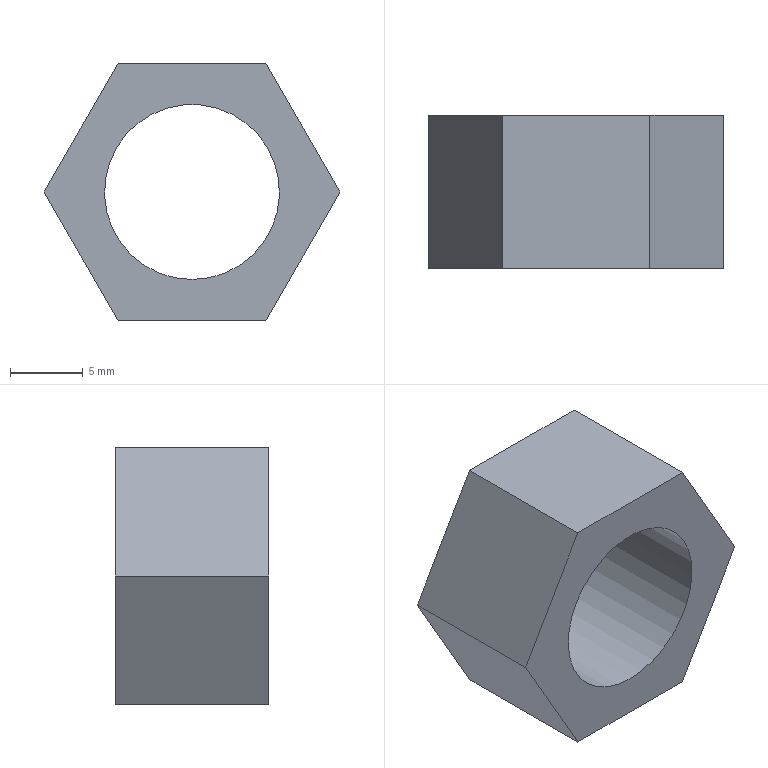Part | NX | features solid 2 | 1 solid | 9 faces | box 20.288 x 10.5 x 17.57 mm | volume 1620 mm3 | plane 8 | cylinder 1 | commonest cylinder face diameters 12 x1
STEP:
#1=CARTESIAN_POINT('',(454.928,470.5,-16.215));
#2=VERTEX_POINT('',#1);
#3=CARTESIAN_POINT('',(449.856,470.5,-25.));
#4=VERTEX_POINT('',#3);
#5=CARTESIAN_POINT('',(454.928,470.5,-16.215));
#6=DIRECTION('',(-0.5,0.,-0.866));
#7=VECTOR('',#6,1000.);
#8=LINE('',#5,#7);
#9=EDGE_CURVE('',#2,#4,#8,.T.);
#10=ORIENTED_EDGE('',*,*,#9,.F.);
#11=CARTESIAN_POINT('',(454.928,481.,-16.215));
#12=VERTEX_POINT('',#11);
#13=CARTESIAN_POINT('',(454.928,481.,-16.215));
#14=DIRECTION('',(0.,-1.,0.));
#15=VECTOR('',#14,1000.);
#16=LINE('',#13,#15);
#17=EDGE_CURVE('',#12,#2,#16,.T.);
#18=ORIENTED_EDGE('',*,*,#17,.F.);
#19=CARTESIAN_POINT('',(449.856,481.,-25.));
#20=VERTEX_POINT('',#19);
#21=CARTESIAN_POINT('',(454.928,481.,-16.215));
#22=DIRECTION('',(-0.5,0.,-0.866));
#23=VECTOR('',#22,1000.);
#24=LINE('',#21,#23);
#25=EDGE_CURVE('',#12,#20,#24,.T.);
#26=ORIENTED_EDGE('',*,*,#25,.T.);
#27=CARTESIAN_POINT('',(449.856,481.,-25.));
#28=DIRECTION('',(0.,-1.,0.));
#29=VECTOR('',#28,1000.);
#30=LINE('',#27,#29);
#31=EDGE_CURVE('',#20,#4,#30,.T.);
#32=ORIENTED_EDGE('',*,*,#31,.T.);
#33=EDGE_LOOP('',(#10,#18,#26,#32));
#34=FACE_BOUND('',#33,.T.);
#35=CARTESIAN_POINT('',(454.928,481.,-16.215));
#36=DIRECTION('',(0.866,0.,-0.5));
#37=DIRECTION('',(0.5,0.,0.866));
#38=AXIS2_PLACEMENT_3D('',#35,#36,#37);
#39=PLANE('',#38);
#40=ADVANCED_FACE('',(#34),#39,.F.);
#41=CARTESIAN_POINT('',(454.928,470.5,-33.785));
#42=VERTEX_POINT('',#41);
#43=CARTESIAN_POINT('',(449.856,470.5,-25.));
#44=DIRECTION('',(0.5,0.,-0.866));
#45=VECTOR('',#44,1000.);
#46=LINE('',#43,#45);
#47=EDGE_CURVE('',#4,#42,#46,.T.);
#48=ORIENTED_EDGE('',*,*,#47,.F.);
#49=ORIENTED_EDGE('',*,*,#31,.F.);
#50=CARTESIAN_POINT('',(454.928,481.,-33.785));
#51=VERTEX_POINT('',#50);
#52=CARTESIAN_POINT('',(449.856,481.,-25.));
#53=DIRECTION('',(0.5,0.,-0.866));
#54=VECTOR('',#53,1000.);
#55=LINE('',#52,#54);
#56=EDGE_CURVE('',#20,#51,#55,.T.);
#57=ORIENTED_EDGE('',*,*,#56,.T.);
#58=CARTESIAN_POINT('',(454.928,481.,-33.785));
#59=DIRECTION('',(0.,-1.,0.));
#60=VECTOR('',#59,1000.);
#61=LINE('',#58,#60);
#62=EDGE_CURVE('',#51,#42,#61,.T.);
#63=ORIENTED_EDGE('',*,*,#62,.T.);
#64=EDGE_LOOP('',(#48,#49,#57,#63));
#65=FACE_BOUND('',#64,.T.);
#66=CARTESIAN_POINT('',(449.856,481.,-25.));
#67=DIRECTION('',(0.866,0.,0.5));
#68=DIRECTION('',(-0.5,0.,0.866));
#69=AXIS2_PLACEMENT_3D('',#66,#67,#68);
#70=PLANE('',#69);
#71=ADVANCED_FACE('',(#65),#70,.F.);
#72=CARTESIAN_POINT('',(465.072,470.5,-33.785));
#73=VERTEX_POINT('',#72);
#74=CARTESIAN_POINT('',(454.928,470.5,-33.785));
#75=DIRECTION('',(1.,0.,0.));
#76=VECTOR('',#75,1000.);
#77=LINE('',#74,#76);
#78=EDGE_CURVE('',#42,#73,#77,.T.);
#79=ORIENTED_EDGE('',*,*,#78,.F.);
#80=ORIENTED_EDGE('',*,*,#62,.F.);
#81=CARTESIAN_POINT('',(465.072,481.,-33.785));
#82=VERTEX_POINT('',#81);
#83=CARTESIAN_POINT('',(454.928,481.,-33.785));
#84=DIRECTION('',(1.,0.,0.));
#85=VECTOR('',#84,1000.);
#86=LINE('',#83,#85);
#87=EDGE_CURVE('',#51,#82,#86,.T.);
#88=ORIENTED_EDGE('',*,*,#87,.T.);
#89=CARTESIAN_POINT('',(465.072,481.,-33.785));
#90=DIRECTION('',(0.,-1.,0.));
#91=VECTOR('',#90,1000.);
#92=LINE('',#89,#91);
#93=EDGE_CURVE('',#82,#73,#92,.T.);
#94=ORIENTED_EDGE('',*,*,#93,.T.);
#95=EDGE_LOOP('',(#79,#80,#88,#94));
#96=FACE_BOUND('',#95,.T.);
#97=CARTESIAN_POINT('',(454.928,481.,-33.785));
#98=DIRECTION('',(0.,0.,1.));
#99=DIRECTION('',(-1.,0.,0.));
#100=AXIS2_PLACEMENT_3D('',#97,#98,#99);
#101=PLANE('',#100);
#102=ADVANCED_FACE('',(#96),#101,.F.);
#103=CARTESIAN_POINT('',(470.144,470.5,-25.));
#104=VERTEX_POINT('',#103);
#105=CARTESIAN_POINT('',(465.072,470.5,-33.785));
#106=DIRECTION('',(0.5,0.,0.866));
#107=VECTOR('',#106,1000.);
#108=LINE('',#105,#107);
#109=EDGE_CURVE('',#73,#104,#108,.T.);
#110=ORIENTED_EDGE('',*,*,#109,.F.);
#111=ORIENTED_EDGE('',*,*,#93,.F.);
#112=CARTESIAN_POINT('',(470.144,481.,-25.));
#113=VERTEX_POINT('',#112);
#114=CARTESIAN_POINT('',(465.072,481.,-33.785));
#115=DIRECTION('',(0.5,0.,0.866));
#116=VECTOR('',#115,1000.);
#117=LINE('',#114,#116);
#118=EDGE_CURVE('',#82,#113,#117,.T.);
#119=ORIENTED_EDGE('',*,*,#118,.T.);
#120=CARTESIAN_POINT('',(470.144,481.,-25.));
#121=DIRECTION('',(0.,-1.,0.));
#122=VECTOR('',#121,1000.);
#123=LINE('',#120,#122);
#124=EDGE_CURVE('',#113,#104,#123,.T.);
#125=ORIENTED_EDGE('',*,*,#124,.T.);
#126=EDGE_LOOP('',(#110,#111,#119,#125));
#127=FACE_BOUND('',#126,.T.);
#128=CARTESIAN_POINT('',(465.072,481.,-33.785));
#129=DIRECTION('',(-0.866,0.,0.5));
#130=DIRECTION('',(-0.5,0.,-0.866));
#131=AXIS2_PLACEMENT_3D('',#128,#129,#130);
#132=PLANE('',#131);
#133=ADVANCED_FACE('',(#127),#132,.F.);
#134=CARTESIAN_POINT('',(465.072,470.5,-16.215));
#135=VERTEX_POINT('',#134);
#136=CARTESIAN_POINT('',(470.144,470.5,-25.));
#137=DIRECTION('',(-0.5,0.,0.866));
#138=VECTOR('',#137,1000.);
#139=LINE('',#136,#138);
#140=EDGE_CURVE('',#104,#135,#139,.T.);
#141=ORIENTED_EDGE('',*,*,#140,.F.);
#142=ORIENTED_EDGE('',*,*,#124,.F.);
#143=CARTESIAN_POINT('',(465.072,481.,-16.215));
#144=VERTEX_POINT('',#143);
#145=CARTESIAN_POINT('',(470.144,481.,-25.));
#146=DIRECTION('',(-0.5,0.,0.866));
#147=VECTOR('',#146,1000.);
#148=LINE('',#145,#147);
#149=EDGE_CURVE('',#113,#144,#148,.T.);
#150=ORIENTED_EDGE('',*,*,#149,.T.);
#151=CARTESIAN_POINT('',(465.072,481.,-16.215));
#152=DIRECTION('',(0.,-1.,0.));
#153=VECTOR('',#152,1000.);
#154=LINE('',#151,#153);
#155=EDGE_CURVE('',#144,#135,#154,.T.);
#156=ORIENTED_EDGE('',*,*,#155,.T.);
#157=EDGE_LOOP('',(#141,#142,#150,#156));
#158=FACE_BOUND('',#157,.T.);
#159=CARTESIAN_POINT('',(470.144,481.,-25.));
#160=DIRECTION('',(-0.866,0.,-0.5));
#161=DIRECTION('',(0.5,0.,-0.866));
#162=AXIS2_PLACEMENT_3D('',#159,#160,#161);
#163=PLANE('',#162);
#164=ADVANCED_FACE('',(#158),#163,.F.);
#165=CARTESIAN_POINT('',(460.,481.,-31.));
#166=VERTEX_POINT('',#165);
#167=CARTESIAN_POINT('',(460.,481.,-25.));
#168=DIRECTION('',(0.,-1.,0.));
#169=DIRECTION('',(0.,0.,-1.));
#170=AXIS2_PLACEMENT_3D('',#167,#168,#169);
#171=CIRCLE('',#170,6.);
#172=EDGE_CURVE('',#166,#166,#171,.T.);
#173=ORIENTED_EDGE('',*,*,#172,.F.);
#174=EDGE_LOOP('',(#173));
#175=FACE_BOUND('',#174,.T.);
#176=CARTESIAN_POINT('',(460.,470.5,-31.));
#177=VERTEX_POINT('',#176);
#178=CARTESIAN_POINT('',(460.,470.5,-25.));
#179=DIRECTION('',(0.,-1.,0.));
#180=DIRECTION('',(0.,0.,-1.));
#181=AXIS2_PLACEMENT_3D('',#178,#179,#180);
#182=CIRCLE('',#181,6.);
#183=EDGE_CURVE('',#177,#177,#182,.T.);
#184=ORIENTED_EDGE('',*,*,#183,.T.);
#185=EDGE_LOOP('',(#184));
#186=FACE_BOUND('',#185,.T.);
#187=CARTESIAN_POINT('',(460.,481.,-25.));
#188=DIRECTION('',(0.,-1.,0.));
#189=DIRECTION('',(0.,0.,1.));
#190=AXIS2_PLACEMENT_3D('',#187,#188,#189);
#191=CYLINDRICAL_SURFACE('',#190,6.);
#192=ADVANCED_FACE('',(#175,#186),#191,.F.);
#193=CARTESIAN_POINT('',(465.072,470.5,-16.215));
#194=DIRECTION('',(-1.,0.,0.));
#195=VECTOR('',#194,1000.);
#196=LINE('',#193,#195);
#197=EDGE_CURVE('',#135,#2,#196,.T.);
#198=ORIENTED_EDGE('',*,*,#197,.F.);
#199=ORIENTED_EDGE('',*,*,#155,.F.);
#200=CARTESIAN_POINT('',(465.072,481.,-16.215));
#201=DIRECTION('',(-1.,0.,0.));
#202=VECTOR('',#201,1000.);
#203=LINE('',#200,#202);
#204=EDGE_CURVE('',#144,#12,#203,.T.);
#205=ORIENTED_EDGE('',*,*,#204,.T.);
#206=ORIENTED_EDGE('',*,*,#17,.T.);
#207=EDGE_LOOP('',(#198,#199,#205,#206));
#208=FACE_BOUND('',#207,.T.);
#209=CARTESIAN_POINT('',(465.072,481.,-16.215));
#210=DIRECTION('',(0.,0.,-1.));
#211=DIRECTION('',(1.,0.,0.));
#212=AXIS2_PLACEMENT_3D('',#209,#210,#211);
#213=PLANE('',#212);
#214=ADVANCED_FACE('',(#208),#213,.F.);
#215=ORIENTED_EDGE('',*,*,#172,.T.);
#216=EDGE_LOOP('',(#215));
#217=FACE_BOUND('',#216,.T.);
#218=ORIENTED_EDGE('',*,*,#25,.F.);
#219=ORIENTED_EDGE('',*,*,#204,.F.);
#220=ORIENTED_EDGE('',*,*,#149,.F.);
#221=ORIENTED_EDGE('',*,*,#118,.F.);
#222=ORIENTED_EDGE('',*,*,#87,.F.);
#223=ORIENTED_EDGE('',*,*,#56,.F.);
#224=EDGE_LOOP('',(#218,#219,#220,#221,#222,#223));
#225=FACE_BOUND('',#224,.T.);
#226=CARTESIAN_POINT('',(444.784,481.,-33.785));
#227=DIRECTION('',(0.,1.,0.));
#228=DIRECTION('',(0.,0.,-1.));
#229=AXIS2_PLACEMENT_3D('',#226,#227,#228);
#230=PLANE('',#229);
#231=ADVANCED_FACE('',(#217,#225),#230,.T.);
#232=ORIENTED_EDGE('',*,*,#183,.F.);
#233=EDGE_LOOP('',(#232));
#234=FACE_BOUND('',#233,.T.);
#235=ORIENTED_EDGE('',*,*,#9,.T.);
#236=ORIENTED_EDGE('',*,*,#47,.T.);
#237=ORIENTED_EDGE('',*,*,#78,.T.);
#238=ORIENTED_EDGE('',*,*,#109,.T.);
#239=ORIENTED_EDGE('',*,*,#140,.T.);
#240=ORIENTED_EDGE('',*,*,#197,.T.);
#241=EDGE_LOOP('',(#235,#236,#237,#238,#239,#240));
#242=FACE_BOUND('',#241,.T.);
#243=CARTESIAN_POINT('',(444.784,470.5,-33.785));
#244=DIRECTION('',(0.,1.,0.));
#245=DIRECTION('',(0.,0.,-1.));
#246=AXIS2_PLACEMENT_3D('',#243,#244,#245);
#247=PLANE('',#246);
#248=ADVANCED_FACE('',(#234,#242),#247,.F.);
#249=CLOSED_SHELL('',(#40,#71,#102,#133,#164,#192,#214,#231,#248));
#250=MANIFOLD_SOLID_BREP('',#249);
#251=(LENGTH_UNIT()NAMED_UNIT(*)SI_UNIT(.MILLI.,.METRE.));
#252=UNCERTAINTY_MEASURE_WITH_UNIT(LENGTH_MEASURE(0.00001),#251,'','');
#253=(NAMED_UNIT(*)PLANE_ANGLE_UNIT()SI_UNIT($,.RADIAN.));
#254=(NAMED_UNIT(*)SI_UNIT($,.STERADIAN.)SOLID_ANGLE_UNIT());
#255=(GEOMETRIC_REPRESENTATION_CONTEXT(3)GLOBAL_UNCERTAINTY_ASSIGNED_CONTEXT((#252))GLOBAL_UNIT_ASSIGNED_CONTEXT((#251,#253,#254))REPRESENTATION_CONTEXT('',''));
#256=ADVANCED_BREP_SHAPE_REPRESENTATION('',(#250),#255);